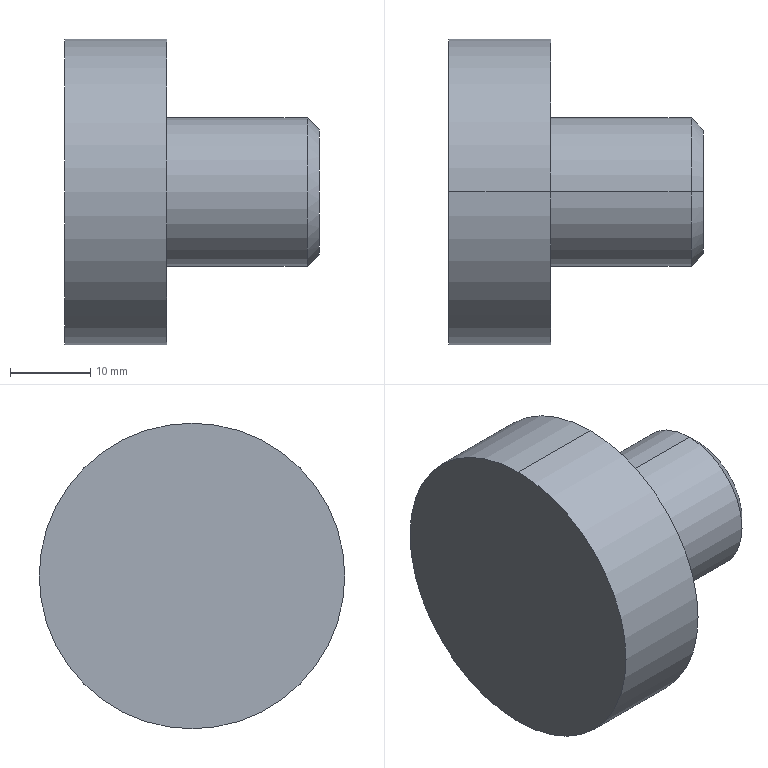Part | SolidWorks | features Revolution 1 | 1 solid | 9 faces | box 31.75 x 38.1 x 38.1 mm | volume 19559 mm3 | cylinder 4 | plane 3 | cone 2 | commonest cylinder face diameters 18.542 x2 38.1 x2
STEP:
#1=CARTESIAN_POINT('',(31.75,0.,7.747));
#2=VERTEX_POINT('',#1);
#3=CARTESIAN_POINT('',(31.75,0.,-7.747));
#4=VERTEX_POINT('',#3);
#5=CARTESIAN_POINT('',(31.75,0.,0.));
#6=DIRECTION('',(-1.,0.,0.));
#7=DIRECTION('',(0.,0.,1.));
#8=AXIS2_PLACEMENT_3D('',#5,#6,#7);
#9=CIRCLE('',#8,7.747);
#10=EDGE_CURVE('',#2,#4,#9,.T.);
#11=ORIENTED_EDGE('',*,*,#10,.T.);
#12=CARTESIAN_POINT('',(30.226,0.,-9.271));
#13=VERTEX_POINT('',#12);
#14=CARTESIAN_POINT('',(31.75,0.,-7.747));
#15=DIRECTION('',(-0.7071,0.,-0.7071));
#16=VECTOR('',#15,1000.);
#17=LINE('',#14,#16);
#18=EDGE_CURVE('',#4,#13,#17,.T.);
#19=ORIENTED_EDGE('',*,*,#18,.T.);
#20=CARTESIAN_POINT('',(30.226,0.,9.271));
#21=VERTEX_POINT('',#20);
#22=CARTESIAN_POINT('',(30.226,0.,0.));
#23=DIRECTION('',(-1.,0.,0.));
#24=DIRECTION('',(0.,0.,1.));
#25=AXIS2_PLACEMENT_3D('',#22,#23,#24);
#26=CIRCLE('',#25,9.271);
#27=EDGE_CURVE('',#21,#13,#26,.T.);
#28=ORIENTED_EDGE('',*,*,#27,.F.);
#29=CARTESIAN_POINT('',(31.75,0.,7.747));
#30=DIRECTION('',(-0.7071,0.,0.7071));
#31=VECTOR('',#30,1000.);
#32=LINE('',#29,#31);
#33=EDGE_CURVE('',#2,#21,#32,.T.);
#34=ORIENTED_EDGE('',*,*,#33,.F.);
#35=EDGE_LOOP('',(#11,#19,#28,#34));
#36=FACE_OUTER_BOUND('',#35,.T.);
#37=CARTESIAN_POINT('',(31.75,0.,0.));
#38=DIRECTION('',(-1.,0.,0.));
#39=DIRECTION('',(0.,0.,1.));
#40=AXIS2_PLACEMENT_3D('',#37,#38,#39);
#41=CONICAL_SURFACE('',#40,7.747,0.7854);
#42=ADVANCED_FACE('',(#36),#41,.T.);
#43=ORIENTED_EDGE('',*,*,#27,.T.);
#44=CARTESIAN_POINT('',(12.7,0.,-9.271));
#45=VERTEX_POINT('',#44);
#46=CARTESIAN_POINT('',(-38.775,0.,-9.271));
#47=DIRECTION('',(-1.,0.,0.));
#48=VECTOR('',#47,1000.);
#49=LINE('',#46,#48);
#50=EDGE_CURVE('',#13,#45,#49,.T.);
#51=ORIENTED_EDGE('',*,*,#50,.T.);
#52=CARTESIAN_POINT('',(12.7,0.,9.271));
#53=VERTEX_POINT('',#52);
#54=CARTESIAN_POINT('',(12.7,0.,0.));
#55=DIRECTION('',(-1.,0.,0.));
#56=DIRECTION('',(0.,0.,1.));
#57=AXIS2_PLACEMENT_3D('',#54,#55,#56);
#58=CIRCLE('',#57,9.271);
#59=EDGE_CURVE('',#53,#45,#58,.T.);
#60=ORIENTED_EDGE('',*,*,#59,.F.);
#61=CARTESIAN_POINT('',(-38.775,0.,9.271));
#62=DIRECTION('',(-1.,0.,0.));
#63=VECTOR('',#62,1000.);
#64=LINE('',#61,#63);
#65=EDGE_CURVE('',#21,#53,#64,.T.);
#66=ORIENTED_EDGE('',*,*,#65,.F.);
#67=EDGE_LOOP('',(#43,#51,#60,#66));
#68=FACE_OUTER_BOUND('',#67,.T.);
#69=CARTESIAN_POINT('',(-38.775,0.,0.));
#70=DIRECTION('',(-1.,0.,0.));
#71=DIRECTION('',(0.,0.,1.));
#72=AXIS2_PLACEMENT_3D('',#69,#70,#71);
#73=CYLINDRICAL_SURFACE('',#72,9.271);
#74=ADVANCED_FACE('',(#68),#73,.T.);
#75=CARTESIAN_POINT('',(12.7,0.,19.05));
#76=VERTEX_POINT('',#75);
#77=CARTESIAN_POINT('',(12.7,0.,-19.05));
#78=VERTEX_POINT('',#77);
#79=CARTESIAN_POINT('',(12.7,0.,0.));
#80=DIRECTION('',(-1.,0.,0.));
#81=DIRECTION('',(0.,0.,1.));
#82=AXIS2_PLACEMENT_3D('',#79,#80,#81);
#83=CIRCLE('',#82,19.05);
#84=EDGE_CURVE('',#76,#78,#83,.T.);
#85=ORIENTED_EDGE('',*,*,#84,.T.);
#86=CARTESIAN_POINT('',(0.,0.,-19.05));
#87=VERTEX_POINT('',#86);
#88=CARTESIAN_POINT('',(-38.775,0.,-19.05));
#89=DIRECTION('',(-1.,0.,0.));
#90=VECTOR('',#89,1000.);
#91=LINE('',#88,#90);
#92=EDGE_CURVE('',#78,#87,#91,.T.);
#93=ORIENTED_EDGE('',*,*,#92,.T.);
#94=CARTESIAN_POINT('',(0.,0.,19.05));
#95=VERTEX_POINT('',#94);
#96=CARTESIAN_POINT('',(0.,0.,0.));
#97=DIRECTION('',(-1.,0.,0.));
#98=DIRECTION('',(0.,0.,1.));
#99=AXIS2_PLACEMENT_3D('',#96,#97,#98);
#100=CIRCLE('',#99,19.05);
#101=EDGE_CURVE('',#95,#87,#100,.T.);
#102=ORIENTED_EDGE('',*,*,#101,.F.);
#103=CARTESIAN_POINT('',(-38.775,0.,19.05));
#104=DIRECTION('',(-1.,0.,0.));
#105=VECTOR('',#104,1000.);
#106=LINE('',#103,#105);
#107=EDGE_CURVE('',#76,#95,#106,.T.);
#108=ORIENTED_EDGE('',*,*,#107,.F.);
#109=EDGE_LOOP('',(#85,#93,#102,#108));
#110=FACE_OUTER_BOUND('',#109,.T.);
#111=CARTESIAN_POINT('',(-38.775,0.,0.));
#112=DIRECTION('',(-1.,0.,0.));
#113=DIRECTION('',(0.,0.,1.));
#114=AXIS2_PLACEMENT_3D('',#111,#112,#113);
#115=CYLINDRICAL_SURFACE('',#114,19.05);
#116=ADVANCED_FACE('',(#110),#115,.T.);
#117=ORIENTED_EDGE('',*,*,#101,.T.);
#118=CARTESIAN_POINT('',(0.,0.,0.));
#119=DIRECTION('',(-1.,0.,0.));
#120=DIRECTION('',(0.,0.,1.));
#121=AXIS2_PLACEMENT_3D('',#118,#119,#120);
#122=CIRCLE('',#121,19.05);
#123=EDGE_CURVE('',#87,#95,#122,.T.);
#124=ORIENTED_EDGE('',*,*,#123,.T.);
#125=EDGE_LOOP('',(#117,#124));
#126=FACE_OUTER_BOUND('',#125,.T.);
#127=CARTESIAN_POINT('',(0.,0.,0.));
#128=DIRECTION('',(1.,0.,0.));
#129=DIRECTION('',(0.,0.,-1.));
#130=AXIS2_PLACEMENT_3D('',#127,#128,#129);
#131=PLANE('',#130);
#132=ADVANCED_FACE('',(#126),#131,.F.);
#133=ORIENTED_EDGE('',*,*,#92,.F.);
#134=CARTESIAN_POINT('',(12.7,0.,0.));
#135=DIRECTION('',(-1.,0.,0.));
#136=DIRECTION('',(0.,0.,1.));
#137=AXIS2_PLACEMENT_3D('',#134,#135,#136);
#138=CIRCLE('',#137,19.05);
#139=EDGE_CURVE('',#78,#76,#138,.T.);
#140=ORIENTED_EDGE('',*,*,#139,.T.);
#141=ORIENTED_EDGE('',*,*,#107,.T.);
#142=ORIENTED_EDGE('',*,*,#123,.F.);
#143=EDGE_LOOP('',(#133,#140,#141,#142));
#144=FACE_OUTER_BOUND('',#143,.T.);
#145=CARTESIAN_POINT('',(-38.775,0.,0.));
#146=DIRECTION('',(-1.,0.,0.));
#147=DIRECTION('',(0.,0.,1.));
#148=AXIS2_PLACEMENT_3D('',#145,#146,#147);
#149=CYLINDRICAL_SURFACE('',#148,19.05);
#150=ADVANCED_FACE('',(#144),#149,.T.);
#151=ORIENTED_EDGE('',*,*,#84,.F.);
#152=ORIENTED_EDGE('',*,*,#139,.F.);
#153=EDGE_LOOP('',(#151,#152));
#154=FACE_OUTER_BOUND('',#153,.T.);
#155=ORIENTED_EDGE('',*,*,#59,.T.);
#156=CARTESIAN_POINT('',(12.7,0.,0.));
#157=DIRECTION('',(-1.,0.,0.));
#158=DIRECTION('',(0.,0.,1.));
#159=AXIS2_PLACEMENT_3D('',#156,#157,#158);
#160=CIRCLE('',#159,9.271);
#161=EDGE_CURVE('',#45,#53,#160,.T.);
#162=ORIENTED_EDGE('',*,*,#161,.T.);
#163=EDGE_LOOP('',(#155,#162));
#164=FACE_BOUND('',#163,.T.);
#165=CARTESIAN_POINT('',(12.7,19.05,0.));
#166=DIRECTION('',(-1.,0.,0.));
#167=DIRECTION('',(0.,0.,1.));
#168=AXIS2_PLACEMENT_3D('',#165,#166,#167);
#169=PLANE('',#168);
#170=ADVANCED_FACE('',(#154,#164),#169,.F.);
#171=ORIENTED_EDGE('',*,*,#50,.F.);
#172=CARTESIAN_POINT('',(30.226,0.,0.));
#173=DIRECTION('',(-1.,0.,0.));
#174=DIRECTION('',(0.,0.,1.));
#175=AXIS2_PLACEMENT_3D('',#172,#173,#174);
#176=CIRCLE('',#175,9.271);
#177=EDGE_CURVE('',#13,#21,#176,.T.);
#178=ORIENTED_EDGE('',*,*,#177,.T.);
#179=ORIENTED_EDGE('',*,*,#65,.T.);
#180=ORIENTED_EDGE('',*,*,#161,.F.);
#181=EDGE_LOOP('',(#171,#178,#179,#180));
#182=FACE_OUTER_BOUND('',#181,.T.);
#183=CARTESIAN_POINT('',(-38.775,0.,0.));
#184=DIRECTION('',(-1.,0.,0.));
#185=DIRECTION('',(0.,0.,1.));
#186=AXIS2_PLACEMENT_3D('',#183,#184,#185);
#187=CYLINDRICAL_SURFACE('',#186,9.271);
#188=ADVANCED_FACE('',(#182),#187,.T.);
#189=ORIENTED_EDGE('',*,*,#18,.F.);
#190=CARTESIAN_POINT('',(31.75,0.,0.));
#191=DIRECTION('',(-1.,0.,0.));
#192=DIRECTION('',(0.,0.,1.));
#193=AXIS2_PLACEMENT_3D('',#190,#191,#192);
#194=CIRCLE('',#193,7.747);
#195=EDGE_CURVE('',#4,#2,#194,.T.);
#196=ORIENTED_EDGE('',*,*,#195,.T.);
#197=ORIENTED_EDGE('',*,*,#33,.T.);
#198=ORIENTED_EDGE('',*,*,#177,.F.);
#199=EDGE_LOOP('',(#189,#196,#197,#198));
#200=FACE_OUTER_BOUND('',#199,.T.);
#201=CARTESIAN_POINT('',(31.75,0.,0.));
#202=DIRECTION('',(-1.,0.,0.));
#203=DIRECTION('',(0.,0.,1.));
#204=AXIS2_PLACEMENT_3D('',#201,#202,#203);
#205=CONICAL_SURFACE('',#204,7.747,0.7854);
#206=ADVANCED_FACE('',(#200),#205,.T.);
#207=ORIENTED_EDGE('',*,*,#10,.F.);
#208=ORIENTED_EDGE('',*,*,#195,.F.);
#209=EDGE_LOOP('',(#207,#208));
#210=FACE_OUTER_BOUND('',#209,.T.);
#211=CARTESIAN_POINT('',(31.75,7.747,0.));
#212=DIRECTION('',(-1.,0.,0.));
#213=DIRECTION('',(0.,0.,1.));
#214=AXIS2_PLACEMENT_3D('',#211,#212,#213);
#215=PLANE('',#214);
#216=ADVANCED_FACE('',(#210),#215,.F.);
#217=CLOSED_SHELL('',(#42,#74,#116,#132,#150,#170,#188,#206,#216));
#218=MANIFOLD_SOLID_BREP('',#217);
#219=CARTESIAN_POINT('',(0.,0.,0.));
#220=DIRECTION('',(0.,0.,1.));
#221=DIRECTION('',(1.,0.,0.));
#222=AXIS2_PLACEMENT_3D('',#219,#220,#221);
#223=(LENGTH_UNIT()NAMED_UNIT(*)SI_UNIT(.MILLI.,.METRE.));
#224=UNCERTAINTY_MEASURE_WITH_UNIT(LENGTH_MEASURE(0.00001),#223,'','');
#225=(NAMED_UNIT(*)PLANE_ANGLE_UNIT()SI_UNIT($,.RADIAN.));
#226=(NAMED_UNIT(*)SI_UNIT($,.STERADIAN.)SOLID_ANGLE_UNIT());
#227=(GEOMETRIC_REPRESENTATION_CONTEXT(3)GLOBAL_UNCERTAINTY_ASSIGNED_CONTEXT((#224))GLOBAL_UNIT_ASSIGNED_CONTEXT((#223,#225,#226))REPRESENTATION_CONTEXT('',''));
#228=ADVANCED_BREP_SHAPE_REPRESENTATION('',(#218,#222),#227);